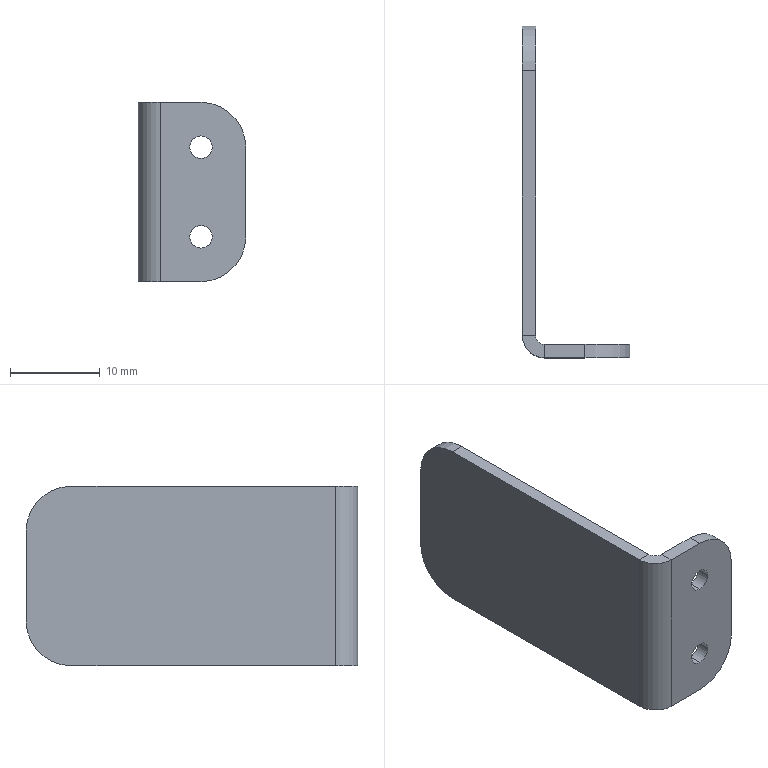Part | SolidWorks | features BreakCorner 1, FlatPattern 1, HoleWzd 1, SMBaseFlange 1, SheetMetal 1 | 1 solid | 22 faces | box 12 x 37 x 20 mm | volume 1356 mm3 | plane 12 | cylinder 10 | commonest cylinder face diameters 2.5 x4 10 x4 2 x1 5 x1
STEP:
#1=CARTESIAN_POINT('',(7.,0.,-6.25));
#2=VERTEX_POINT('',#1);
#3=CARTESIAN_POINT('',(7.,0.,-3.75));
#4=VERTEX_POINT('',#3);
#5=CARTESIAN_POINT('',(7.,0.,-5.));
#6=DIRECTION('',(0.,1.,0.));
#7=DIRECTION('',(0.,0.,1.));
#8=AXIS2_PLACEMENT_3D('',#5,#6,#7);
#9=CIRCLE('',#8,1.25);
#10=EDGE_CURVE('',#2,#4,#9,.T.);
#11=ORIENTED_EDGE('',*,*,#10,.F.);
#12=CARTESIAN_POINT('',(7.,1.5,-6.25));
#13=VERTEX_POINT('',#12);
#14=CARTESIAN_POINT('',(7.,1.5,-6.25));
#15=DIRECTION('',(0.,1.,0.));
#16=VECTOR('',#15,1000.);
#17=LINE('',#14,#16);
#18=EDGE_CURVE('',#2,#13,#17,.T.);
#19=ORIENTED_EDGE('',*,*,#18,.T.);
#20=CARTESIAN_POINT('',(7.,1.5,-3.75));
#21=VERTEX_POINT('',#20);
#22=CARTESIAN_POINT('',(7.,1.5,-5.));
#23=DIRECTION('',(0.,1.,0.));
#24=DIRECTION('',(0.,0.,1.));
#25=AXIS2_PLACEMENT_3D('',#22,#23,#24);
#26=CIRCLE('',#25,1.25);
#27=EDGE_CURVE('',#13,#21,#26,.T.);
#28=ORIENTED_EDGE('',*,*,#27,.T.);
#29=CARTESIAN_POINT('',(7.,1.5,-3.75));
#30=DIRECTION('',(0.,1.,0.));
#31=VECTOR('',#30,1000.);
#32=LINE('',#29,#31);
#33=EDGE_CURVE('',#4,#21,#32,.T.);
#34=ORIENTED_EDGE('',*,*,#33,.F.);
#35=EDGE_LOOP('',(#11,#19,#28,#34));
#36=FACE_OUTER_BOUND('',#35,.T.);
#37=CARTESIAN_POINT('',(7.,1.5,-5.));
#38=DIRECTION('',(0.,1.,0.));
#39=DIRECTION('',(0.,0.,1.));
#40=AXIS2_PLACEMENT_3D('',#37,#38,#39);
#41=CYLINDRICAL_SURFACE('',#40,1.25);
#42=ADVANCED_FACE('',(#36),#41,.F.);
#43=CARTESIAN_POINT('',(7.,0.,3.75));
#44=VERTEX_POINT('',#43);
#45=CARTESIAN_POINT('',(7.,0.,6.25));
#46=VERTEX_POINT('',#45);
#47=CARTESIAN_POINT('',(7.,0.,5.));
#48=DIRECTION('',(0.,1.,0.));
#49=DIRECTION('',(0.,0.,1.));
#50=AXIS2_PLACEMENT_3D('',#47,#48,#49);
#51=CIRCLE('',#50,1.25);
#52=EDGE_CURVE('',#44,#46,#51,.T.);
#53=ORIENTED_EDGE('',*,*,#52,.F.);
#54=CARTESIAN_POINT('',(7.,1.5,3.75));
#55=VERTEX_POINT('',#54);
#56=CARTESIAN_POINT('',(7.,1.5,3.75));
#57=DIRECTION('',(0.,1.,0.));
#58=VECTOR('',#57,1000.);
#59=LINE('',#56,#58);
#60=EDGE_CURVE('',#44,#55,#59,.T.);
#61=ORIENTED_EDGE('',*,*,#60,.T.);
#62=CARTESIAN_POINT('',(7.,1.5,6.25));
#63=VERTEX_POINT('',#62);
#64=CARTESIAN_POINT('',(7.,1.5,5.));
#65=DIRECTION('',(0.,1.,0.));
#66=DIRECTION('',(0.,0.,1.));
#67=AXIS2_PLACEMENT_3D('',#64,#65,#66);
#68=CIRCLE('',#67,1.25);
#69=EDGE_CURVE('',#55,#63,#68,.T.);
#70=ORIENTED_EDGE('',*,*,#69,.T.);
#71=CARTESIAN_POINT('',(7.,1.5,6.25));
#72=DIRECTION('',(0.,1.,0.));
#73=VECTOR('',#72,1000.);
#74=LINE('',#71,#73);
#75=EDGE_CURVE('',#46,#63,#74,.T.);
#76=ORIENTED_EDGE('',*,*,#75,.F.);
#77=EDGE_LOOP('',(#53,#61,#70,#76));
#78=FACE_OUTER_BOUND('',#77,.T.);
#79=CARTESIAN_POINT('',(7.,1.5,5.));
#80=DIRECTION('',(0.,1.,0.));
#81=DIRECTION('',(0.,0.,1.));
#82=AXIS2_PLACEMENT_3D('',#79,#80,#81);
#83=CYLINDRICAL_SURFACE('',#82,1.25);
#84=ADVANCED_FACE('',(#78),#83,.F.);
#85=CARTESIAN_POINT('',(0.,2.5,10.));
#86=VERTEX_POINT('',#85);
#87=CARTESIAN_POINT('',(1.5,2.5,10.));
#88=VERTEX_POINT('',#87);
#89=CARTESIAN_POINT('',(0.,2.5,10.));
#90=DIRECTION('',(1.,0.,0.));
#91=VECTOR('',#90,1000.);
#92=LINE('',#89,#91);
#93=EDGE_CURVE('',#86,#88,#92,.T.);
#94=ORIENTED_EDGE('',*,*,#93,.F.);
#95=CARTESIAN_POINT('',(2.5,0.,10.));
#96=VERTEX_POINT('',#95);
#97=CARTESIAN_POINT('',(2.5,2.5,10.));
#98=DIRECTION('',(0.,0.,1.));
#99=DIRECTION('',(-1.,0.,0.));
#100=AXIS2_PLACEMENT_3D('',#97,#98,#99);
#101=CIRCLE('',#100,2.5);
#102=EDGE_CURVE('',#86,#96,#101,.T.);
#103=ORIENTED_EDGE('',*,*,#102,.T.);
#104=CARTESIAN_POINT('',(2.5,1.5,10.));
#105=VERTEX_POINT('',#104);
#106=CARTESIAN_POINT('',(2.5,1.5,10.));
#107=DIRECTION('',(0.,-1.,0.));
#108=VECTOR('',#107,1000.);
#109=LINE('',#106,#108);
#110=EDGE_CURVE('',#105,#96,#109,.T.);
#111=ORIENTED_EDGE('',*,*,#110,.F.);
#112=CARTESIAN_POINT('',(2.5,2.5,10.));
#113=DIRECTION('',(0.,0.,1.));
#114=DIRECTION('',(1.,0.,0.));
#115=AXIS2_PLACEMENT_3D('',#112,#113,#114);
#116=CIRCLE('',#115,1.);
#117=EDGE_CURVE('',#88,#105,#116,.T.);
#118=ORIENTED_EDGE('',*,*,#117,.F.);
#119=EDGE_LOOP('',(#94,#103,#111,#118));
#120=FACE_OUTER_BOUND('',#119,.T.);
#121=CARTESIAN_POINT('',(0.,2.5,10.));
#122=DIRECTION('',(0.,0.,1.));
#123=DIRECTION('',(1.,0.,0.));
#124=AXIS2_PLACEMENT_3D('',#121,#122,#123);
#125=PLANE('',#124);
#126=ADVANCED_FACE('',(#120),#125,.T.);
#127=CARTESIAN_POINT('',(1.5,32.,10.));
#128=VERTEX_POINT('',#127);
#129=CARTESIAN_POINT('',(1.5,37.,10.));
#130=DIRECTION('',(0.,-1.,0.));
#131=VECTOR('',#130,1000.);
#132=LINE('',#129,#131);
#133=EDGE_CURVE('',#128,#88,#132,.T.);
#134=ORIENTED_EDGE('',*,*,#133,.F.);
#135=CARTESIAN_POINT('',(0.,32.,10.));
#136=VERTEX_POINT('',#135);
#137=CARTESIAN_POINT('',(2.5,32.,10.));
#138=DIRECTION('',(-1.,0.,0.));
#139=VECTOR('',#138,1000.);
#140=LINE('',#137,#139);
#141=EDGE_CURVE('',#128,#136,#140,.T.);
#142=ORIENTED_EDGE('',*,*,#141,.T.);
#143=CARTESIAN_POINT('',(0.,37.,10.));
#144=DIRECTION('',(0.,-1.,0.));
#145=VECTOR('',#144,1000.);
#146=LINE('',#143,#145);
#147=EDGE_CURVE('',#136,#86,#146,.T.);
#148=ORIENTED_EDGE('',*,*,#147,.T.);
#149=ORIENTED_EDGE('',*,*,#93,.T.);
#150=EDGE_LOOP('',(#134,#142,#148,#149));
#151=FACE_OUTER_BOUND('',#150,.T.);
#152=CARTESIAN_POINT('',(2.5,1.5,10.));
#153=DIRECTION('',(0.,0.,1.));
#154=DIRECTION('',(1.,0.,0.));
#155=AXIS2_PLACEMENT_3D('',#152,#153,#154);
#156=PLANE('',#155);
#157=ADVANCED_FACE('',(#151),#156,.T.);
#158=CARTESIAN_POINT('',(2.5,0.,-10.));
#159=VERTEX_POINT('',#158);
#160=CARTESIAN_POINT('',(2.5,1.5,-10.));
#161=VERTEX_POINT('',#160);
#162=CARTESIAN_POINT('',(2.5,0.,-10.));
#163=DIRECTION('',(0.,1.,0.));
#164=VECTOR('',#163,1000.);
#165=LINE('',#162,#164);
#166=EDGE_CURVE('',#159,#161,#165,.T.);
#167=ORIENTED_EDGE('',*,*,#166,.F.);
#168=CARTESIAN_POINT('',(0.,2.5,-10.));
#169=VERTEX_POINT('',#168);
#170=CARTESIAN_POINT('',(2.5,2.5,-10.));
#171=DIRECTION('',(0.,0.,1.));
#172=DIRECTION('',(-1.,0.,0.));
#173=AXIS2_PLACEMENT_3D('',#170,#171,#172);
#174=CIRCLE('',#173,2.5);
#175=EDGE_CURVE('',#169,#159,#174,.T.);
#176=ORIENTED_EDGE('',*,*,#175,.F.);
#177=CARTESIAN_POINT('',(1.5,2.5,-10.));
#178=VERTEX_POINT('',#177);
#179=CARTESIAN_POINT('',(1.5,2.5,-10.));
#180=DIRECTION('',(-1.,0.,0.));
#181=VECTOR('',#180,1000.);
#182=LINE('',#179,#181);
#183=EDGE_CURVE('',#178,#169,#182,.T.);
#184=ORIENTED_EDGE('',*,*,#183,.F.);
#185=CARTESIAN_POINT('',(2.5,2.5,-10.));
#186=DIRECTION('',(0.,0.,1.));
#187=DIRECTION('',(1.,0.,0.));
#188=AXIS2_PLACEMENT_3D('',#185,#186,#187);
#189=CIRCLE('',#188,1.);
#190=EDGE_CURVE('',#178,#161,#189,.T.);
#191=ORIENTED_EDGE('',*,*,#190,.T.);
#192=EDGE_LOOP('',(#167,#176,#184,#191));
#193=FACE_OUTER_BOUND('',#192,.T.);
#194=CARTESIAN_POINT('',(2.5,0.,-10.));
#195=DIRECTION('',(0.,0.,-1.));
#196=DIRECTION('',(-1.,0.,0.));
#197=AXIS2_PLACEMENT_3D('',#194,#195,#196);
#198=PLANE('',#197);
#199=ADVANCED_FACE('',(#193),#198,.T.);
#200=CARTESIAN_POINT('',(7.,1.5,-10.));
#201=VERTEX_POINT('',#200);
#202=CARTESIAN_POINT('',(0.,1.5,-10.));
#203=DIRECTION('',(1.,0.,0.));
#204=VECTOR('',#203,1000.);
#205=LINE('',#202,#204);
#206=EDGE_CURVE('',#161,#201,#205,.T.);
#207=ORIENTED_EDGE('',*,*,#206,.T.);
#208=CARTESIAN_POINT('',(7.,0.,-10.));
#209=VERTEX_POINT('',#208);
#210=CARTESIAN_POINT('',(7.,2.5,-10.));
#211=DIRECTION('',(0.,-1.,0.));
#212=VECTOR('',#211,1000.);
#213=LINE('',#210,#212);
#214=EDGE_CURVE('',#201,#209,#213,.T.);
#215=ORIENTED_EDGE('',*,*,#214,.T.);
#216=CARTESIAN_POINT('',(0.,0.,-10.));
#217=DIRECTION('',(1.,0.,0.));
#218=VECTOR('',#217,1000.);
#219=LINE('',#216,#218);
#220=EDGE_CURVE('',#159,#209,#219,.T.);
#221=ORIENTED_EDGE('',*,*,#220,.F.);
#222=ORIENTED_EDGE('',*,*,#166,.T.);
#223=EDGE_LOOP('',(#207,#215,#221,#222));
#224=FACE_OUTER_BOUND('',#223,.T.);
#225=CARTESIAN_POINT('',(1.5,2.5,-10.));
#226=DIRECTION('',(0.,0.,-1.));
#227=DIRECTION('',(-1.,0.,0.));
#228=AXIS2_PLACEMENT_3D('',#225,#226,#227);
#229=PLANE('',#228);
#230=ADVANCED_FACE('',(#224),#229,.T.);
#231=CARTESIAN_POINT('',(7.,0.,-5.));
#232=DIRECTION('',(0.,1.,0.));
#233=DIRECTION('',(0.,0.,1.));
#234=AXIS2_PLACEMENT_3D('',#231,#232,#233);
#235=CIRCLE('',#234,1.25);
#236=EDGE_CURVE('',#4,#2,#235,.T.);
#237=ORIENTED_EDGE('',*,*,#236,.T.);
#238=ORIENTED_EDGE('',*,*,#10,.T.);
#239=EDGE_LOOP('',(#237,#238));
#240=FACE_BOUND('',#239,.T.);
#241=CARTESIAN_POINT('',(7.,0.,5.));
#242=DIRECTION('',(0.,1.,0.));
#243=DIRECTION('',(0.,0.,1.));
#244=AXIS2_PLACEMENT_3D('',#241,#242,#243);
#245=CIRCLE('',#244,1.25);
#246=EDGE_CURVE('',#46,#44,#245,.T.);
#247=ORIENTED_EDGE('',*,*,#246,.T.);
#248=ORIENTED_EDGE('',*,*,#52,.T.);
#249=EDGE_LOOP('',(#247,#248));
#250=FACE_BOUND('',#249,.T.);
#251=CARTESIAN_POINT('',(12.,0.,5.));
#252=VERTEX_POINT('',#251);
#253=CARTESIAN_POINT('',(12.,0.,-5.));
#254=VERTEX_POINT('',#253);
#255=CARTESIAN_POINT('',(12.,0.,10.));
#256=DIRECTION('',(0.,0.,-1.));
#257=VECTOR('',#256,1000.);
#258=LINE('',#255,#257);
#259=EDGE_CURVE('',#252,#254,#258,.T.);
#260=ORIENTED_EDGE('',*,*,#259,.F.);
#261=CARTESIAN_POINT('',(7.,0.,10.));
#262=VERTEX_POINT('',#261);
#263=CARTESIAN_POINT('',(7.,0.,5.));
#264=DIRECTION('',(0.,-1.,0.));
#265=DIRECTION('',(0.,0.,1.));
#266=AXIS2_PLACEMENT_3D('',#263,#264,#265);
#267=CIRCLE('',#266,5.);
#268=EDGE_CURVE('',#252,#262,#267,.T.);
#269=ORIENTED_EDGE('',*,*,#268,.T.);
#270=CARTESIAN_POINT('',(0.,0.,10.));
#271=DIRECTION('',(1.,0.,0.));
#272=VECTOR('',#271,1000.);
#273=LINE('',#270,#272);
#274=EDGE_CURVE('',#96,#262,#273,.T.);
#275=ORIENTED_EDGE('',*,*,#274,.F.);
#276=CARTESIAN_POINT('',(2.5,0.,10.));
#277=DIRECTION('',(0.,0.,-1.));
#278=VECTOR('',#277,1000.);
#279=LINE('',#276,#278);
#280=EDGE_CURVE('',#96,#159,#279,.T.);
#281=ORIENTED_EDGE('',*,*,#280,.T.);
#282=ORIENTED_EDGE('',*,*,#220,.T.);
#283=CARTESIAN_POINT('',(7.,0.,-5.));
#284=DIRECTION('',(0.,-1.,0.));
#285=DIRECTION('',(0.,0.,1.));
#286=AXIS2_PLACEMENT_3D('',#283,#284,#285);
#287=CIRCLE('',#286,5.);
#288=EDGE_CURVE('',#209,#254,#287,.T.);
#289=ORIENTED_EDGE('',*,*,#288,.T.);
#290=EDGE_LOOP('',(#260,#269,#275,#281,#282,#289));
#291=FACE_OUTER_BOUND('',#290,.T.);
#292=CARTESIAN_POINT('',(0.,0.,10.));
#293=DIRECTION('',(0.,1.,0.));
#294=DIRECTION('',(0.,0.,1.));
#295=AXIS2_PLACEMENT_3D('',#292,#293,#294);
#296=PLANE('',#295);
#297=ADVANCED_FACE('',(#240,#250,#291),#296,.F.);
#298=CARTESIAN_POINT('',(12.,1.5,5.));
#299=VERTEX_POINT('',#298);
#300=CARTESIAN_POINT('',(12.,1.5,-5.));
#301=VERTEX_POINT('',#300);
#302=CARTESIAN_POINT('',(12.,1.5,10.));
#303=DIRECTION('',(0.,0.,-1.));
#304=VECTOR('',#303,1000.);
#305=LINE('',#302,#304);
#306=EDGE_CURVE('',#299,#301,#305,.T.);
#307=ORIENTED_EDGE('',*,*,#306,.F.);
#308=CARTESIAN_POINT('',(12.,1.5,5.));
#309=DIRECTION('',(0.,-1.,0.));
#310=VECTOR('',#309,1000.);
#311=LINE('',#308,#310);
#312=EDGE_CURVE('',#299,#252,#311,.T.);
#313=ORIENTED_EDGE('',*,*,#312,.T.);
#314=ORIENTED_EDGE('',*,*,#259,.T.);
#315=CARTESIAN_POINT('',(12.,1.5,-5.));
#316=DIRECTION('',(0.,1.,0.));
#317=VECTOR('',#316,1000.);
#318=LINE('',#315,#317);
#319=EDGE_CURVE('',#254,#301,#318,.T.);
#320=ORIENTED_EDGE('',*,*,#319,.T.);
#321=EDGE_LOOP('',(#307,#313,#314,#320));
#322=FACE_OUTER_BOUND('',#321,.T.);
#323=CARTESIAN_POINT('',(12.,1.5,10.));
#324=DIRECTION('',(1.,0.,0.));
#325=DIRECTION('',(0.,0.,-1.));
#326=AXIS2_PLACEMENT_3D('',#323,#324,#325);
#327=PLANE('',#326);
#328=ADVANCED_FACE('',(#322),#327,.T.);
#329=CARTESIAN_POINT('',(7.,1.5,-5.));
#330=DIRECTION('',(0.,1.,0.));
#331=DIRECTION('',(0.,0.,1.));
#332=AXIS2_PLACEMENT_3D('',#329,#330,#331);
#333=CIRCLE('',#332,1.25);
#334=EDGE_CURVE('',#21,#13,#333,.T.);
#335=ORIENTED_EDGE('',*,*,#334,.F.);
#336=ORIENTED_EDGE('',*,*,#27,.F.);
#337=EDGE_LOOP('',(#335,#336));
#338=FACE_BOUND('',#337,.T.);
#339=CARTESIAN_POINT('',(7.,1.5,5.));
#340=DIRECTION('',(0.,1.,0.));
#341=DIRECTION('',(0.,0.,1.));
#342=AXIS2_PLACEMENT_3D('',#339,#340,#341);
#343=CIRCLE('',#342,1.25);
#344=EDGE_CURVE('',#63,#55,#343,.T.);
#345=ORIENTED_EDGE('',*,*,#344,.F.);
#346=ORIENTED_EDGE('',*,*,#69,.F.);
#347=EDGE_LOOP('',(#345,#346));
#348=FACE_BOUND('',#347,.T.);
#349=CARTESIAN_POINT('',(7.,1.5,10.));
#350=VERTEX_POINT('',#349);
#351=CARTESIAN_POINT('',(0.,1.5,10.));
#352=DIRECTION('',(1.,0.,0.));
#353=VECTOR('',#352,1000.);
#354=LINE('',#351,#353);
#355=EDGE_CURVE('',#105,#350,#354,.T.);
#356=ORIENTED_EDGE('',*,*,#355,.T.);
#357=CARTESIAN_POINT('',(7.,1.5,5.));
#358=DIRECTION('',(0.,1.,0.));
#359=DIRECTION('',(0.,0.,1.));
#360=AXIS2_PLACEMENT_3D('',#357,#358,#359);
#361=CIRCLE('',#360,5.);
#362=EDGE_CURVE('',#350,#299,#361,.T.);
#363=ORIENTED_EDGE('',*,*,#362,.T.);
#364=ORIENTED_EDGE('',*,*,#306,.T.);
#365=CARTESIAN_POINT('',(7.,1.5,-5.));
#366=DIRECTION('',(0.,1.,0.));
#367=DIRECTION('',(0.,0.,1.));
#368=AXIS2_PLACEMENT_3D('',#365,#366,#367);
#369=CIRCLE('',#368,5.);
#370=EDGE_CURVE('',#301,#201,#369,.T.);
#371=ORIENTED_EDGE('',*,*,#370,.T.);
#372=ORIENTED_EDGE('',*,*,#206,.F.);
#373=CARTESIAN_POINT('',(2.5,1.5,10.));
#374=DIRECTION('',(0.,0.,-1.));
#375=VECTOR('',#374,1000.);
#376=LINE('',#373,#375);
#377=EDGE_CURVE('',#105,#161,#376,.T.);
#378=ORIENTED_EDGE('',*,*,#377,.F.);
#379=EDGE_LOOP('',(#356,#363,#364,#371,#372,#378));
#380=FACE_OUTER_BOUND('',#379,.T.);
#381=CARTESIAN_POINT('',(0.,1.5,10.));
#382=DIRECTION('',(0.,1.,0.));
#383=DIRECTION('',(0.,0.,1.));
#384=AXIS2_PLACEMENT_3D('',#381,#382,#383);
#385=PLANE('',#384);
#386=ADVANCED_FACE('',(#338,#348,#380),#385,.T.);
#387=ORIENTED_EDGE('',*,*,#190,.F.);
#388=CARTESIAN_POINT('',(1.5,2.5,10.));
#389=DIRECTION('',(0.,0.,-1.));
#390=VECTOR('',#389,1000.);
#391=LINE('',#388,#390);
#392=EDGE_CURVE('',#88,#178,#391,.T.);
#393=ORIENTED_EDGE('',*,*,#392,.F.);
#394=ORIENTED_EDGE('',*,*,#117,.T.);
#395=ORIENTED_EDGE('',*,*,#377,.T.);
#396=EDGE_LOOP('',(#387,#393,#394,#395));
#397=FACE_OUTER_BOUND('',#396,.T.);
#398=CARTESIAN_POINT('',(2.5,2.5,10.));
#399=DIRECTION('',(0.,0.,-1.));
#400=DIRECTION('',(-1.,0.,0.));
#401=AXIS2_PLACEMENT_3D('',#398,#399,#400);
#402=CYLINDRICAL_SURFACE('',#401,1.);
#403=ADVANCED_FACE('',(#397),#402,.F.);
#404=CARTESIAN_POINT('',(1.5,37.,5.));
#405=VERTEX_POINT('',#404);
#406=CARTESIAN_POINT('',(1.5,37.,-5.));
#407=VERTEX_POINT('',#406);
#408=CARTESIAN_POINT('',(1.5,37.,10.));
#409=DIRECTION('',(0.,0.,-1.));
#410=VECTOR('',#409,1000.);
#411=LINE('',#408,#410);
#412=EDGE_CURVE('',#405,#407,#411,.T.);
#413=ORIENTED_EDGE('',*,*,#412,.F.);
#414=CARTESIAN_POINT('',(1.5,32.,5.));
#415=DIRECTION('',(1.,0.,0.));
#416=DIRECTION('',(0.,1.,0.));
#417=AXIS2_PLACEMENT_3D('',#414,#415,#416);
#418=CIRCLE('',#417,5.);
#419=EDGE_CURVE('',#405,#128,#418,.T.);
#420=ORIENTED_EDGE('',*,*,#419,.T.);
#421=ORIENTED_EDGE('',*,*,#133,.T.);
#422=ORIENTED_EDGE('',*,*,#392,.T.);
#423=CARTESIAN_POINT('',(1.5,32.,-10.));
#424=VERTEX_POINT('',#423);
#425=CARTESIAN_POINT('',(1.5,37.,-10.));
#426=DIRECTION('',(0.,-1.,0.));
#427=VECTOR('',#426,1000.);
#428=LINE('',#425,#427);
#429=EDGE_CURVE('',#424,#178,#428,.T.);
#430=ORIENTED_EDGE('',*,*,#429,.F.);
#431=CARTESIAN_POINT('',(1.5,32.,-5.));
#432=DIRECTION('',(1.,0.,0.));
#433=DIRECTION('',(0.,1.,0.));
#434=AXIS2_PLACEMENT_3D('',#431,#432,#433);
#435=CIRCLE('',#434,5.);
#436=EDGE_CURVE('',#424,#407,#435,.T.);
#437=ORIENTED_EDGE('',*,*,#436,.T.);
#438=EDGE_LOOP('',(#413,#420,#421,#422,#430,#437));
#439=FACE_OUTER_BOUND('',#438,.T.);
#440=CARTESIAN_POINT('',(1.5,37.,10.));
#441=DIRECTION('',(1.,0.,0.));
#442=DIRECTION('',(0.,1.,0.));
#443=AXIS2_PLACEMENT_3D('',#440,#441,#442);
#444=PLANE('',#443);
#445=ADVANCED_FACE('',(#439),#444,.T.);
#446=CARTESIAN_POINT('',(0.,37.,5.));
#447=VERTEX_POINT('',#446);
#448=CARTESIAN_POINT('',(0.,37.,-5.));
#449=VERTEX_POINT('',#448);
#450=CARTESIAN_POINT('',(0.,37.,10.));
#451=DIRECTION('',(0.,0.,-1.));
#452=VECTOR('',#451,1000.);
#453=LINE('',#450,#452);
#454=EDGE_CURVE('',#447,#449,#453,.T.);
#455=ORIENTED_EDGE('',*,*,#454,.F.);
#456=CARTESIAN_POINT('',(0.,37.,5.));
#457=DIRECTION('',(1.,0.,0.));
#458=VECTOR('',#457,1000.);
#459=LINE('',#456,#458);
#460=EDGE_CURVE('',#447,#405,#459,.T.);
#461=ORIENTED_EDGE('',*,*,#460,.T.);
#462=ORIENTED_EDGE('',*,*,#412,.T.);
#463=CARTESIAN_POINT('',(0.,37.,-5.));
#464=DIRECTION('',(-1.,0.,0.));
#465=VECTOR('',#464,1000.);
#466=LINE('',#463,#465);
#467=EDGE_CURVE('',#407,#449,#466,.T.);
#468=ORIENTED_EDGE('',*,*,#467,.T.);
#469=EDGE_LOOP('',(#455,#461,#462,#468));
#470=FACE_OUTER_BOUND('',#469,.T.);
#471=CARTESIAN_POINT('',(0.,37.,10.));
#472=DIRECTION('',(0.,1.,0.));
#473=DIRECTION('',(0.,0.,1.));
#474=AXIS2_PLACEMENT_3D('',#471,#472,#473);
#475=PLANE('',#474);
#476=ADVANCED_FACE('',(#470),#475,.T.);
#477=ORIENTED_EDGE('',*,*,#147,.F.);
#478=CARTESIAN_POINT('',(0.,32.,5.));
#479=DIRECTION('',(-1.,0.,0.));
#480=DIRECTION('',(0.,1.,0.));
#481=AXIS2_PLACEMENT_3D('',#478,#479,#480);
#482=CIRCLE('',#481,5.);
#483=EDGE_CURVE('',#136,#447,#482,.T.);
#484=ORIENTED_EDGE('',*,*,#483,.T.);
#485=ORIENTED_EDGE('',*,*,#454,.T.);
#486=CARTESIAN_POINT('',(0.,32.,-10.));
#487=VERTEX_POINT('',#486);
#488=CARTESIAN_POINT('',(0.,32.,-5.));
#489=DIRECTION('',(-1.,0.,0.));
#490=DIRECTION('',(0.,1.,0.));
#491=AXIS2_PLACEMENT_3D('',#488,#489,#490);
#492=CIRCLE('',#491,5.);
#493=EDGE_CURVE('',#449,#487,#492,.T.);
#494=ORIENTED_EDGE('',*,*,#493,.T.);
#495=CARTESIAN_POINT('',(0.,37.,-10.));
#496=DIRECTION('',(0.,-1.,0.));
#497=VECTOR('',#496,1000.);
#498=LINE('',#495,#497);
#499=EDGE_CURVE('',#487,#169,#498,.T.);
#500=ORIENTED_EDGE('',*,*,#499,.T.);
#501=CARTESIAN_POINT('',(0.,2.5,10.));
#502=DIRECTION('',(0.,0.,-1.));
#503=VECTOR('',#502,1000.);
#504=LINE('',#501,#503);
#505=EDGE_CURVE('',#86,#169,#504,.T.);
#506=ORIENTED_EDGE('',*,*,#505,.F.);
#507=EDGE_LOOP('',(#477,#484,#485,#494,#500,#506));
#508=FACE_OUTER_BOUND('',#507,.T.);
#509=CARTESIAN_POINT('',(0.,37.,10.));
#510=DIRECTION('',(1.,0.,0.));
#511=DIRECTION('',(0.,1.,0.));
#512=AXIS2_PLACEMENT_3D('',#509,#510,#511);
#513=PLANE('',#512);
#514=ADVANCED_FACE('',(#508),#513,.F.);
#515=ORIENTED_EDGE('',*,*,#175,.T.);
#516=ORIENTED_EDGE('',*,*,#280,.F.);
#517=ORIENTED_EDGE('',*,*,#102,.F.);
#518=ORIENTED_EDGE('',*,*,#505,.T.);
#519=EDGE_LOOP('',(#515,#516,#517,#518));
#520=FACE_OUTER_BOUND('',#519,.T.);
#521=CARTESIAN_POINT('',(2.5,2.5,10.));
#522=DIRECTION('',(0.,0.,-1.));
#523=DIRECTION('',(-1.,0.,0.));
#524=AXIS2_PLACEMENT_3D('',#521,#522,#523);
#525=CYLINDRICAL_SURFACE('',#524,2.5);
#526=ADVANCED_FACE('',(#520),#525,.T.);
#527=ORIENTED_EDGE('',*,*,#274,.T.);
#528=CARTESIAN_POINT('',(7.,2.5,10.));
#529=DIRECTION('',(0.,1.,0.));
#530=VECTOR('',#529,1000.);
#531=LINE('',#528,#530);
#532=EDGE_CURVE('',#262,#350,#531,.T.);
#533=ORIENTED_EDGE('',*,*,#532,.T.);
#534=ORIENTED_EDGE('',*,*,#355,.F.);
#535=ORIENTED_EDGE('',*,*,#110,.T.);
#536=EDGE_LOOP('',(#527,#533,#534,#535));
#537=FACE_OUTER_BOUND('',#536,.T.);
#538=CARTESIAN_POINT('',(2.5,2.5,10.));
#539=DIRECTION('',(0.,0.,1.));
#540=DIRECTION('',(1.,0.,0.));
#541=AXIS2_PLACEMENT_3D('',#538,#539,#540);
#542=PLANE('',#541);
#543=ADVANCED_FACE('',(#537),#542,.T.);
#544=ORIENTED_EDGE('',*,*,#499,.F.);
#545=CARTESIAN_POINT('',(1.5,32.,-10.));
#546=DIRECTION('',(1.,0.,0.));
#547=VECTOR('',#546,1000.);
#548=LINE('',#545,#547);
#549=EDGE_CURVE('',#487,#424,#548,.T.);
#550=ORIENTED_EDGE('',*,*,#549,.T.);
#551=ORIENTED_EDGE('',*,*,#429,.T.);
#552=ORIENTED_EDGE('',*,*,#183,.T.);
#553=EDGE_LOOP('',(#544,#550,#551,#552));
#554=FACE_OUTER_BOUND('',#553,.T.);
#555=CARTESIAN_POINT('',(2.5,2.5,-10.));
#556=DIRECTION('',(0.,0.,1.));
#557=DIRECTION('',(1.,0.,0.));
#558=AXIS2_PLACEMENT_3D('',#555,#556,#557);
#559=PLANE('',#558);
#560=ADVANCED_FACE('',(#554),#559,.F.);
#561=ORIENTED_EDGE('',*,*,#483,.F.);
#562=ORIENTED_EDGE('',*,*,#141,.F.);
#563=ORIENTED_EDGE('',*,*,#419,.F.);
#564=ORIENTED_EDGE('',*,*,#460,.F.);
#565=EDGE_LOOP('',(#561,#562,#563,#564));
#566=FACE_OUTER_BOUND('',#565,.T.);
#567=CARTESIAN_POINT('',(0.,32.,5.));
#568=DIRECTION('',(1.,0.,0.));
#569=DIRECTION('',(0.,0.,-1.));
#570=AXIS2_PLACEMENT_3D('',#567,#568,#569);
#571=CYLINDRICAL_SURFACE('',#570,5.);
#572=ADVANCED_FACE('',(#566),#571,.T.);
#573=ORIENTED_EDGE('',*,*,#493,.F.);
#574=ORIENTED_EDGE('',*,*,#467,.F.);
#575=ORIENTED_EDGE('',*,*,#436,.F.);
#576=ORIENTED_EDGE('',*,*,#549,.F.);
#577=EDGE_LOOP('',(#573,#574,#575,#576));
#578=FACE_OUTER_BOUND('',#577,.T.);
#579=CARTESIAN_POINT('',(2.5,32.,-5.));
#580=DIRECTION('',(-1.,0.,0.));
#581=DIRECTION('',(0.,0.,1.));
#582=AXIS2_PLACEMENT_3D('',#579,#580,#581);
#583=CYLINDRICAL_SURFACE('',#582,5.);
#584=ADVANCED_FACE('',(#578),#583,.T.);
#585=ORIENTED_EDGE('',*,*,#362,.F.);
#586=ORIENTED_EDGE('',*,*,#532,.F.);
#587=ORIENTED_EDGE('',*,*,#268,.F.);
#588=ORIENTED_EDGE('',*,*,#312,.F.);
#589=EDGE_LOOP('',(#585,#586,#587,#588));
#590=FACE_OUTER_BOUND('',#589,.T.);
#591=CARTESIAN_POINT('',(7.,1.5,5.));
#592=DIRECTION('',(0.,-1.,0.));
#593=DIRECTION('',(0.,0.,-1.));
#594=AXIS2_PLACEMENT_3D('',#591,#592,#593);
#595=CYLINDRICAL_SURFACE('',#594,5.);
#596=ADVANCED_FACE('',(#590),#595,.T.);
#597=ORIENTED_EDGE('',*,*,#370,.F.);
#598=ORIENTED_EDGE('',*,*,#319,.F.);
#599=ORIENTED_EDGE('',*,*,#288,.F.);
#600=ORIENTED_EDGE('',*,*,#214,.F.);
#601=EDGE_LOOP('',(#597,#598,#599,#600));
#602=FACE_OUTER_BOUND('',#601,.T.);
#603=CARTESIAN_POINT('',(7.,2.5,-5.));
#604=DIRECTION('',(0.,-1.,0.));
#605=DIRECTION('',(0.,0.,-1.));
#606=AXIS2_PLACEMENT_3D('',#603,#604,#605);
#607=CYLINDRICAL_SURFACE('',#606,5.);
#608=ADVANCED_FACE('',(#602),#607,.T.);
#609=ORIENTED_EDGE('',*,*,#60,.F.);
#610=ORIENTED_EDGE('',*,*,#246,.F.);
#611=ORIENTED_EDGE('',*,*,#75,.T.);
#612=ORIENTED_EDGE('',*,*,#344,.T.);
#613=EDGE_LOOP('',(#609,#610,#611,#612));
#614=FACE_OUTER_BOUND('',#613,.T.);
#615=CARTESIAN_POINT('',(7.,1.5,5.));
#616=DIRECTION('',(0.,1.,0.));
#617=DIRECTION('',(0.,0.,1.));
#618=AXIS2_PLACEMENT_3D('',#615,#616,#617);
#619=CYLINDRICAL_SURFACE('',#618,1.25);
#620=ADVANCED_FACE('',(#614),#619,.F.);
#621=ORIENTED_EDGE('',*,*,#18,.F.);
#622=ORIENTED_EDGE('',*,*,#236,.F.);
#623=ORIENTED_EDGE('',*,*,#33,.T.);
#624=ORIENTED_EDGE('',*,*,#334,.T.);
#625=EDGE_LOOP('',(#621,#622,#623,#624));
#626=FACE_OUTER_BOUND('',#625,.T.);
#627=CARTESIAN_POINT('',(7.,1.5,-5.));
#628=DIRECTION('',(0.,1.,0.));
#629=DIRECTION('',(0.,0.,1.));
#630=AXIS2_PLACEMENT_3D('',#627,#628,#629);
#631=CYLINDRICAL_SURFACE('',#630,1.25);
#632=ADVANCED_FACE('',(#626),#631,.F.);
#633=CLOSED_SHELL('',(#42,#84,#126,#157,#199,#230,#297,#328,#386,#403,#445,#476,#514,#526,#543,#560,#572,#584,#596,#608,#620,#632));
#634=MANIFOLD_SOLID_BREP('',#633);
#635=CARTESIAN_POINT('',(0.,0.,0.));
#636=DIRECTION('',(0.,0.,1.));
#637=DIRECTION('',(1.,0.,0.));
#638=AXIS2_PLACEMENT_3D('',#635,#636,#637);
#639=(LENGTH_UNIT()NAMED_UNIT(*)SI_UNIT(.MILLI.,.METRE.));
#640=UNCERTAINTY_MEASURE_WITH_UNIT(LENGTH_MEASURE(0.00001),#639,'','');
#641=(NAMED_UNIT(*)PLANE_ANGLE_UNIT()SI_UNIT($,.RADIAN.));
#642=(NAMED_UNIT(*)SI_UNIT($,.STERADIAN.)SOLID_ANGLE_UNIT());
#643=(GEOMETRIC_REPRESENTATION_CONTEXT(3)GLOBAL_UNCERTAINTY_ASSIGNED_CONTEXT((#640))GLOBAL_UNIT_ASSIGNED_CONTEXT((#639,#641,#642))REPRESENTATION_CONTEXT('',''));
#644=ADVANCED_BREP_SHAPE_REPRESENTATION('',(#634,#638),#643);